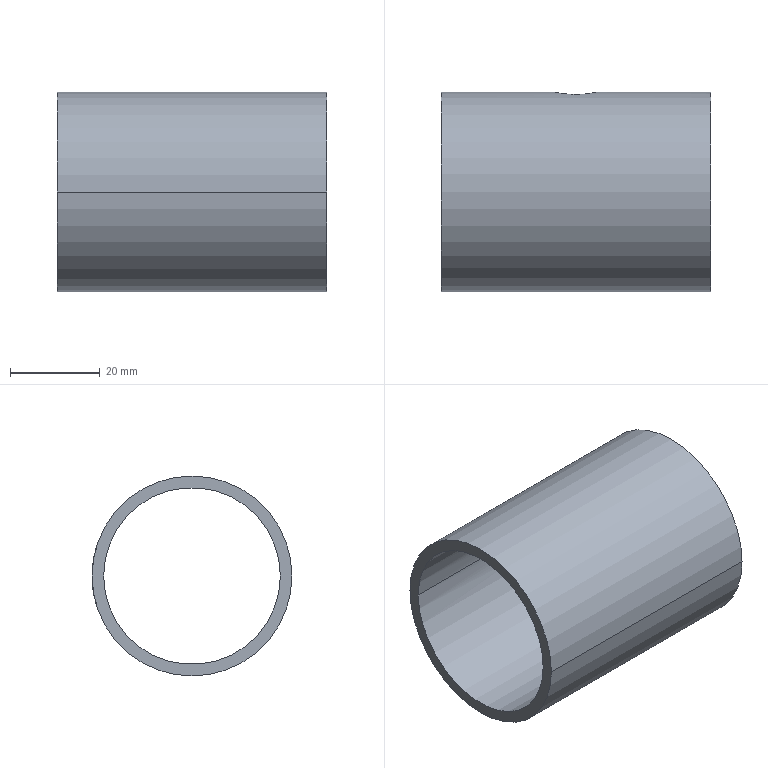Part | NX | features BREP 1 | 1 solid | 8 faces | box 59.944 x 44.45 x 44.45 mm | volume 20229 mm3 | cylinder 6 | plane 2 | commonest cylinder face diameters 9.779 x2 39.268 x2 44.45 x2
STEP:
#1=CARTESIAN_POINT('',(-29.972,22.225,0.));
#2=VERTEX_POINT('',#1);
#3=CARTESIAN_POINT('',(-29.972,-22.225,0.));
#4=VERTEX_POINT('',#3);
#5=CARTESIAN_POINT('',(-29.972,0.,0.));
#6=DIRECTION('',(1.,0.,0.));
#7=DIRECTION('',(0.,1.,0.));
#8=AXIS2_PLACEMENT_3D('',#5,#6,#7);
#9=CIRCLE('',#8,22.225);
#10=EDGE_CURVE('',#2,#4,#9,.T.);
#11=ORIENTED_EDGE('',*,*,#10,.F.);
#12=CARTESIAN_POINT('',(-29.972,0.,0.));
#13=DIRECTION('',(1.,0.,0.));
#14=DIRECTION('',(0.,-1.,0.));
#15=AXIS2_PLACEMENT_3D('',#12,#13,#14);
#16=CIRCLE('',#15,22.225);
#17=EDGE_CURVE('',#4,#2,#16,.T.);
#18=ORIENTED_EDGE('',*,*,#17,.F.);
#19=EDGE_LOOP('',(#11,#18));
#20=FACE_BOUND('',#19,.T.);
#21=CARTESIAN_POINT('',(-29.972,19.634,0.));
#22=VERTEX_POINT('',#21);
#23=CARTESIAN_POINT('',(-29.972,-19.634,0.));
#24=VERTEX_POINT('',#23);
#25=CARTESIAN_POINT('',(-29.972,0.,0.));
#26=DIRECTION('',(-1.,0.,0.));
#27=DIRECTION('',(0.,1.,0.));
#28=AXIS2_PLACEMENT_3D('',#25,#26,#27);
#29=CIRCLE('',#28,19.634);
#30=EDGE_CURVE('',#22,#24,#29,.T.);
#31=ORIENTED_EDGE('',*,*,#30,.F.);
#32=CARTESIAN_POINT('',(-29.972,0.,0.));
#33=DIRECTION('',(-1.,0.,0.));
#34=DIRECTION('',(0.,-1.,0.));
#35=AXIS2_PLACEMENT_3D('',#32,#33,#34);
#36=CIRCLE('',#35,19.634);
#37=EDGE_CURVE('',#24,#22,#36,.T.);
#38=ORIENTED_EDGE('',*,*,#37,.F.);
#39=EDGE_LOOP('',(#31,#38));
#40=FACE_BOUND('',#39,.T.);
#41=CARTESIAN_POINT('',(-29.972,0.,0.));
#42=DIRECTION('',(1.,0.,0.));
#43=DIRECTION('',(0.,1.,0.));
#44=AXIS2_PLACEMENT_3D('',#41,#42,#43);
#45=PLANE('',#44);
#46=ADVANCED_FACE('',(#20,#40),#45,.F.);
#47=CARTESIAN_POINT('',(4.889,22.225,0.));
#48=VERTEX_POINT('',#47);
#49=CARTESIAN_POINT('',(29.972,22.225,0.));
#50=VERTEX_POINT('',#49);
#51=CARTESIAN_POINT('',(4.889,22.225,0.));
#52=DIRECTION('',(1.,0.,0.));
#53=VECTOR('',#52,1000.);
#54=LINE('',#51,#53);
#55=EDGE_CURVE('',#48,#50,#54,.T.);
#56=ORIENTED_EDGE('',*,*,#55,.T.);
#57=CARTESIAN_POINT('',(29.972,-22.225,0.));
#58=VERTEX_POINT('',#57);
#59=CARTESIAN_POINT('',(29.972,0.,0.));
#60=DIRECTION('',(1.,0.,0.));
#61=DIRECTION('',(0.,-1.,0.));
#62=AXIS2_PLACEMENT_3D('',#59,#60,#61);
#63=CIRCLE('',#62,22.225);
#64=EDGE_CURVE('',#58,#50,#63,.T.);
#65=ORIENTED_EDGE('',*,*,#64,.F.);
#66=CARTESIAN_POINT('',(-29.972,-22.225,0.));
#67=DIRECTION('',(1.,0.,0.));
#68=VECTOR('',#67,1000.);
#69=LINE('',#66,#68);
#70=EDGE_CURVE('',#58,#4,#69,.F.);
#71=ORIENTED_EDGE('',*,*,#70,.T.);
#72=ORIENTED_EDGE('',*,*,#17,.T.);
#73=CARTESIAN_POINT('',(-4.889,22.225,0.));
#74=VERTEX_POINT('',#73);
#75=CARTESIAN_POINT('',(-29.972,22.225,0.));
#76=DIRECTION('',(1.,0.,0.));
#77=VECTOR('',#76,1000.);
#78=LINE('',#75,#77);
#79=EDGE_CURVE('',#74,#2,#78,.F.);
#80=ORIENTED_EDGE('',*,*,#79,.F.);
#81=CARTESIAN_POINT('',(-4.889,22.225,0.));
#82=CARTESIAN_POINT('',(-4.889,22.225,-1.282));
#83=CARTESIAN_POINT('',(-3.851,21.961,-3.8));
#84=CARTESIAN_POINT('',(-0.02854,21.542,-5.426));
#85=CARTESIAN_POINT('',(3.829,21.955,-3.833));
#86=CARTESIAN_POINT('',(4.889,22.225,-1.294));
#87=CARTESIAN_POINT('',(4.889,22.225,0.));
#88=B_SPLINE_CURVE_WITH_KNOTS('',3,(#81,#82,#83,#84,#85,#86,#87),.UNSPECIFIED.,.F.,.F.,(4,1,1,1,4),(0.,0.25,0.5,0.75,1.),.UNSPECIFIED.);
#89=EDGE_CURVE('',#74,#48,#88,.T.);
#90=ORIENTED_EDGE('',*,*,#89,.T.);
#91=EDGE_LOOP('',(#56,#65,#71,#72,#80,#90));
#92=FACE_BOUND('',#91,.T.);
#93=CARTESIAN_POINT('',(-29.972,0.,0.));
#94=DIRECTION('',(1.,0.,0.));
#95=DIRECTION('',(0.,-1.,0.));
#96=AXIS2_PLACEMENT_3D('',#93,#94,#95);
#97=CYLINDRICAL_SURFACE('',#96,22.225);
#98=ADVANCED_FACE('',(#92),#97,.T.);
#99=CARTESIAN_POINT('',(-4.889,19.634,0.));
#100=VERTEX_POINT('',#99);
#101=CARTESIAN_POINT('',(-4.889,22.225,0.));
#102=DIRECTION('',(0.,-1.,0.));
#103=VECTOR('',#102,1000.);
#104=LINE('',#101,#103);
#105=EDGE_CURVE('',#74,#100,#104,.T.);
#106=ORIENTED_EDGE('',*,*,#105,.T.);
#107=CARTESIAN_POINT('',(4.889,19.634,0.));
#108=VERTEX_POINT('',#107);
#109=CARTESIAN_POINT('',(-4.889,19.634,0.));
#110=CARTESIAN_POINT('',(-4.889,19.634,-0.3023));
#111=CARTESIAN_POINT('',(-4.841,19.621,-0.9094));
#112=CARTESIAN_POINT('',(-4.581,19.559,-1.751));
#113=CARTESIAN_POINT('',(-4.346,19.505,-2.259));
#114=CARTESIAN_POINT('',(-4.057,19.443,-2.741));
#115=CARTESIAN_POINT('',(-3.865,19.404,-3.004));
#116=CARTESIAN_POINT('',(-3.492,19.332,-3.445));
#117=CARTESIAN_POINT('',(-3.009,19.252,-3.862));
#118=CARTESIAN_POINT('',(-2.789,19.218,-4.024));
#119=CARTESIAN_POINT('',(-2.291,19.152,-4.33));
#120=CARTESIAN_POINT('',(-1.797,19.097,-4.562));
#121=CARTESIAN_POINT('',(-0.9325,19.03,-4.838));
#122=CARTESIAN_POINT('',(-0.02377,19.009,-4.913));
#123=CARTESIAN_POINT('',(0.8917,19.028,-4.846));
#124=CARTESIAN_POINT('',(1.751,19.093,-4.581));
#125=CARTESIAN_POINT('',(2.255,19.147,-4.349));
#126=CARTESIAN_POINT('',(2.753,19.213,-4.049));
#127=CARTESIAN_POINT('',(2.989,19.248,-3.877));
#128=CARTESIAN_POINT('',(3.466,19.327,-3.471));
#129=CARTESIAN_POINT('',(3.854,19.401,-3.019));
#130=CARTESIAN_POINT('',(4.042,19.44,-2.763));
#131=CARTESIAN_POINT('',(4.338,19.504,-2.275));
#132=CARTESIAN_POINT('',(4.575,19.558,-1.766));
#133=CARTESIAN_POINT('',(4.84,19.621,-0.9161));
#134=CARTESIAN_POINT('',(4.889,19.634,-0.3045));
#135=CARTESIAN_POINT('',(4.889,19.634,0.));
#136=B_SPLINE_CURVE_WITH_KNOTS('',3,(#109,#110,#111,#112,#113,#114,#115,#116,#117,#118,#119,#120,#121,#122,#123,#124,#125,#126,#127,#128,#129,#130,#131,#132,#133,#134,#135),.UNSPECIFIED.,.F.,.F.,(4,1,1,1,1,1,1,1,1,1,1,1,1,1,1,1,1,1,1,1,1,1,1,1,4),(0.,0.0625,0.125,0.1562,0.1875,0.2188,0.25,0.2812,0.3125,0.3438,0.375,0.4375,0.5,0.5625,0.625,0.6562,0.6875,0.7188,0.75,0.7812,0.8125,0.8438,0.875,0.9375,1.),.UNSPECIFIED.);
#137=EDGE_CURVE('',#108,#100,#136,.F.);
#138=ORIENTED_EDGE('',*,*,#137,.F.);
#139=CARTESIAN_POINT('',(4.889,22.225,0.));
#140=DIRECTION('',(0.,-1.,0.));
#141=VECTOR('',#140,1000.);
#142=LINE('',#139,#141);
#143=EDGE_CURVE('',#48,#108,#142,.T.);
#144=ORIENTED_EDGE('',*,*,#143,.F.);
#145=ORIENTED_EDGE('',*,*,#89,.F.);
#146=EDGE_LOOP('',(#106,#138,#144,#145));
#147=FACE_BOUND('',#146,.T.);
#148=CARTESIAN_POINT('',(0.,22.225,0.));
#149=DIRECTION('',(0.,1.,0.));
#150=DIRECTION('',(1.,0.,0.));
#151=AXIS2_PLACEMENT_3D('',#148,#149,#150);
#152=CYLINDRICAL_SURFACE('',#151,4.889);
#153=ADVANCED_FACE('',(#147),#152,.F.);
#154=ORIENTED_EDGE('',*,*,#143,.T.);
#155=CARTESIAN_POINT('',(4.889,19.634,0.));
#156=CARTESIAN_POINT('',(4.889,19.634,0.3025));
#157=CARTESIAN_POINT('',(4.841,19.621,0.9101));
#158=CARTESIAN_POINT('',(4.58,19.559,1.753));
#159=CARTESIAN_POINT('',(4.345,19.505,2.261));
#160=CARTESIAN_POINT('',(4.056,19.443,2.744));
#161=CARTESIAN_POINT('',(3.863,19.403,3.005));
#162=CARTESIAN_POINT('',(3.489,19.331,3.448));
#163=CARTESIAN_POINT('',(3.007,19.251,3.864));
#164=CARTESIAN_POINT('',(2.785,19.217,4.026));
#165=CARTESIAN_POINT('',(2.287,19.151,4.332));
#166=CARTESIAN_POINT('',(1.792,19.097,4.565));
#167=CARTESIAN_POINT('',(0.9283,19.03,4.839));
#168=CARTESIAN_POINT('',(0.01934,19.009,4.913));
#169=CARTESIAN_POINT('',(-0.8952,19.028,4.845));
#170=CARTESIAN_POINT('',(-1.754,19.093,4.579));
#171=CARTESIAN_POINT('',(-2.257,19.147,4.348));
#172=CARTESIAN_POINT('',(-2.756,19.213,4.047));
#173=CARTESIAN_POINT('',(-2.99,19.249,3.876));
#174=CARTESIAN_POINT('',(-3.468,19.327,3.47));
#175=CARTESIAN_POINT('',(-3.854,19.402,3.018));
#176=CARTESIAN_POINT('',(-4.043,19.44,2.762));
#177=CARTESIAN_POINT('',(-4.339,19.504,2.274));
#178=CARTESIAN_POINT('',(-4.576,19.558,1.765));
#179=CARTESIAN_POINT('',(-4.84,19.621,0.9157));
#180=CARTESIAN_POINT('',(-4.889,19.634,0.3044));
#181=CARTESIAN_POINT('',(-4.889,19.634,0.));
#182=B_SPLINE_CURVE_WITH_KNOTS('',3,(#155,#156,#157,#158,#159,#160,#161,#162,#163,#164,#165,#166,#167,#168,#169,#170,#171,#172,#173,#174,#175,#176,#177,#178,#179,#180,#181),.UNSPECIFIED.,.F.,.F.,(4,1,1,1,1,1,1,1,1,1,1,1,1,1,1,1,1,1,1,1,1,1,1,1,4),(0.,0.0625,0.125,0.1562,0.1875,0.2188,0.25,0.2812,0.3125,0.3438,0.375,0.4375,0.5,0.5625,0.625,0.6562,0.6875,0.7188,0.75,0.7812,0.8125,0.8438,0.875,0.9375,1.),.UNSPECIFIED.);
#183=EDGE_CURVE('',#100,#108,#182,.F.);
#184=ORIENTED_EDGE('',*,*,#183,.F.);
#185=ORIENTED_EDGE('',*,*,#105,.F.);
#186=CARTESIAN_POINT('',(-4.889,22.225,0.));
#187=CARTESIAN_POINT('',(-4.889,22.225,0.3041));
#188=CARTESIAN_POINT('',(-4.841,22.213,0.9148));
#189=CARTESIAN_POINT('',(-4.576,22.158,1.764));
#190=CARTESIAN_POINT('',(-4.34,22.11,2.273));
#191=CARTESIAN_POINT('',(-4.043,22.054,2.762));
#192=CARTESIAN_POINT('',(-3.857,22.02,3.015));
#193=CARTESIAN_POINT('',(-3.465,21.954,3.472));
#194=CARTESIAN_POINT('',(-2.998,21.886,3.87));
#195=CARTESIAN_POINT('',(-2.752,21.853,4.05));
#196=CARTESIAN_POINT('',(-2.254,21.796,4.349));
#197=CARTESIAN_POINT('',(-1.754,21.748,4.58));
#198=CARTESIAN_POINT('',(-0.8943,21.692,4.845));
#199=CARTESIAN_POINT('',(0.01906,21.675,4.913));
#200=CARTESIAN_POINT('',(0.9289,21.693,4.839));
#201=CARTESIAN_POINT('',(1.79,21.751,4.565));
#202=CARTESIAN_POINT('',(2.286,21.799,4.333));
#203=CARTESIAN_POINT('',(2.783,21.857,4.028));
#204=CARTESIAN_POINT('',(3.009,21.888,3.862));
#205=CARTESIAN_POINT('',(3.488,21.957,3.449));
#206=CARTESIAN_POINT('',(3.865,22.022,3.004));
#207=CARTESIAN_POINT('',(4.055,22.056,2.744));
#208=CARTESIAN_POINT('',(4.346,22.111,2.26));
#209=CARTESIAN_POINT('',(4.581,22.159,1.752));
#210=CARTESIAN_POINT('',(4.841,22.213,0.9094));
#211=CARTESIAN_POINT('',(4.889,22.225,0.3022));
#212=CARTESIAN_POINT('',(4.889,22.225,0.));
#213=B_SPLINE_CURVE_WITH_KNOTS('',3,(#186,#187,#188,#189,#190,#191,#192,#193,#194,#195,#196,#197,#198,#199,#200,#201,#202,#203,#204,#205,#206,#207,#208,#209,#210,#211,#212),.UNSPECIFIED.,.F.,.F.,(4,1,1,1,1,1,1,1,1,1,1,1,1,1,1,1,1,1,1,1,1,1,1,1,4),(0.,0.0625,0.125,0.1562,0.1875,0.2188,0.25,0.2812,0.3125,0.3438,0.375,0.4375,0.5,0.5625,0.625,0.6562,0.6875,0.7188,0.75,0.7812,0.8125,0.8438,0.875,0.9375,1.),.UNSPECIFIED.);
#214=EDGE_CURVE('',#48,#74,#213,.F.);
#215=ORIENTED_EDGE('',*,*,#214,.F.);
#216=EDGE_LOOP('',(#154,#184,#185,#215));
#217=FACE_BOUND('',#216,.T.);
#218=CARTESIAN_POINT('',(0.,22.225,0.));
#219=DIRECTION('',(0.,1.,0.));
#220=DIRECTION('',(1.,0.,0.));
#221=AXIS2_PLACEMENT_3D('',#218,#219,#220);
#222=CYLINDRICAL_SURFACE('',#221,4.889);
#223=ADVANCED_FACE('',(#217),#222,.F.);
#224=ORIENTED_EDGE('',*,*,#79,.T.);
#225=ORIENTED_EDGE('',*,*,#10,.T.);
#226=ORIENTED_EDGE('',*,*,#70,.F.);
#227=CARTESIAN_POINT('',(29.972,0.,0.));
#228=DIRECTION('',(1.,0.,0.));
#229=DIRECTION('',(0.,1.,0.));
#230=AXIS2_PLACEMENT_3D('',#227,#228,#229);
#231=CIRCLE('',#230,22.225);
#232=EDGE_CURVE('',#50,#58,#231,.T.);
#233=ORIENTED_EDGE('',*,*,#232,.F.);
#234=ORIENTED_EDGE('',*,*,#55,.F.);
#235=ORIENTED_EDGE('',*,*,#214,.T.);
#236=EDGE_LOOP('',(#224,#225,#226,#233,#234,#235));
#237=FACE_BOUND('',#236,.T.);
#238=CARTESIAN_POINT('',(-29.972,0.,0.));
#239=DIRECTION('',(1.,0.,0.));
#240=DIRECTION('',(0.,-1.,0.));
#241=AXIS2_PLACEMENT_3D('',#238,#239,#240);
#242=CYLINDRICAL_SURFACE('',#241,22.225);
#243=ADVANCED_FACE('',(#237),#242,.T.);
#244=ORIENTED_EDGE('',*,*,#232,.T.);
#245=ORIENTED_EDGE('',*,*,#64,.T.);
#246=EDGE_LOOP('',(#244,#245));
#247=FACE_BOUND('',#246,.T.);
#248=CARTESIAN_POINT('',(29.972,19.634,0.));
#249=VERTEX_POINT('',#248);
#250=CARTESIAN_POINT('',(29.972,-19.634,0.));
#251=VERTEX_POINT('',#250);
#252=CARTESIAN_POINT('',(29.972,0.,0.));
#253=DIRECTION('',(-1.,0.,0.));
#254=DIRECTION('',(0.,1.,0.));
#255=AXIS2_PLACEMENT_3D('',#252,#253,#254);
#256=CIRCLE('',#255,19.634);
#257=EDGE_CURVE('',#249,#251,#256,.T.);
#258=ORIENTED_EDGE('',*,*,#257,.T.);
#259=CARTESIAN_POINT('',(29.972,0.,0.));
#260=DIRECTION('',(-1.,0.,0.));
#261=DIRECTION('',(0.,-1.,0.));
#262=AXIS2_PLACEMENT_3D('',#259,#260,#261);
#263=CIRCLE('',#262,19.634);
#264=EDGE_CURVE('',#251,#249,#263,.T.);
#265=ORIENTED_EDGE('',*,*,#264,.T.);
#266=EDGE_LOOP('',(#258,#265));
#267=FACE_BOUND('',#266,.T.);
#268=CARTESIAN_POINT('',(29.972,0.,0.));
#269=DIRECTION('',(1.,0.,0.));
#270=DIRECTION('',(0.,1.,0.));
#271=AXIS2_PLACEMENT_3D('',#268,#269,#270);
#272=PLANE('',#271);
#273=ADVANCED_FACE('',(#247,#267),#272,.T.);
#274=CARTESIAN_POINT('',(4.889,19.634,0.));
#275=DIRECTION('',(1.,0.,0.));
#276=VECTOR('',#275,1000.);
#277=LINE('',#274,#276);
#278=EDGE_CURVE('',#108,#249,#277,.T.);
#279=ORIENTED_EDGE('',*,*,#278,.T.);
#280=ORIENTED_EDGE('',*,*,#264,.F.);
#281=CARTESIAN_POINT('',(-29.972,-19.634,0.));
#282=DIRECTION('',(1.,0.,0.));
#283=VECTOR('',#282,1000.);
#284=LINE('',#281,#283);
#285=EDGE_CURVE('',#251,#24,#284,.F.);
#286=ORIENTED_EDGE('',*,*,#285,.T.);
#287=ORIENTED_EDGE('',*,*,#37,.T.);
#288=CARTESIAN_POINT('',(-29.972,19.634,0.));
#289=DIRECTION('',(1.,0.,0.));
#290=VECTOR('',#289,1000.);
#291=LINE('',#288,#290);
#292=EDGE_CURVE('',#100,#22,#291,.F.);
#293=ORIENTED_EDGE('',*,*,#292,.F.);
#294=ORIENTED_EDGE('',*,*,#183,.T.);
#295=EDGE_LOOP('',(#279,#280,#286,#287,#293,#294));
#296=FACE_BOUND('',#295,.T.);
#297=CARTESIAN_POINT('',(-29.972,0.,0.));
#298=DIRECTION('',(1.,0.,0.));
#299=DIRECTION('',(0.,-1.,0.));
#300=AXIS2_PLACEMENT_3D('',#297,#298,#299);
#301=CYLINDRICAL_SURFACE('',#300,19.634);
#302=ADVANCED_FACE('',(#296),#301,.F.);
#303=ORIENTED_EDGE('',*,*,#292,.T.);
#304=ORIENTED_EDGE('',*,*,#30,.T.);
#305=ORIENTED_EDGE('',*,*,#285,.F.);
#306=ORIENTED_EDGE('',*,*,#257,.F.);
#307=ORIENTED_EDGE('',*,*,#278,.F.);
#308=ORIENTED_EDGE('',*,*,#137,.T.);
#309=EDGE_LOOP('',(#303,#304,#305,#306,#307,#308));
#310=FACE_BOUND('',#309,.T.);
#311=CARTESIAN_POINT('',(-29.972,0.,0.));
#312=DIRECTION('',(1.,0.,0.));
#313=DIRECTION('',(0.,-1.,0.));
#314=AXIS2_PLACEMENT_3D('',#311,#312,#313);
#315=CYLINDRICAL_SURFACE('',#314,19.634);
#316=ADVANCED_FACE('',(#310),#315,.F.);
#317=CLOSED_SHELL('',(#46,#98,#153,#223,#243,#273,#302,#316));
#318=MANIFOLD_SOLID_BREP('',#317);
#319=(LENGTH_UNIT()NAMED_UNIT(*)SI_UNIT(.MILLI.,.METRE.));
#320=UNCERTAINTY_MEASURE_WITH_UNIT(LENGTH_MEASURE(0.0508),#319,'','');
#321=(NAMED_UNIT(*)PLANE_ANGLE_UNIT()SI_UNIT($,.RADIAN.));
#322=(NAMED_UNIT(*)SI_UNIT($,.STERADIAN.)SOLID_ANGLE_UNIT());
#323=(GEOMETRIC_REPRESENTATION_CONTEXT(3)GLOBAL_UNCERTAINTY_ASSIGNED_CONTEXT((#320))GLOBAL_UNIT_ASSIGNED_CONTEXT((#319,#321,#322))REPRESENTATION_CONTEXT('',''));
#324=ADVANCED_BREP_SHAPE_REPRESENTATION('',(#318),#323);